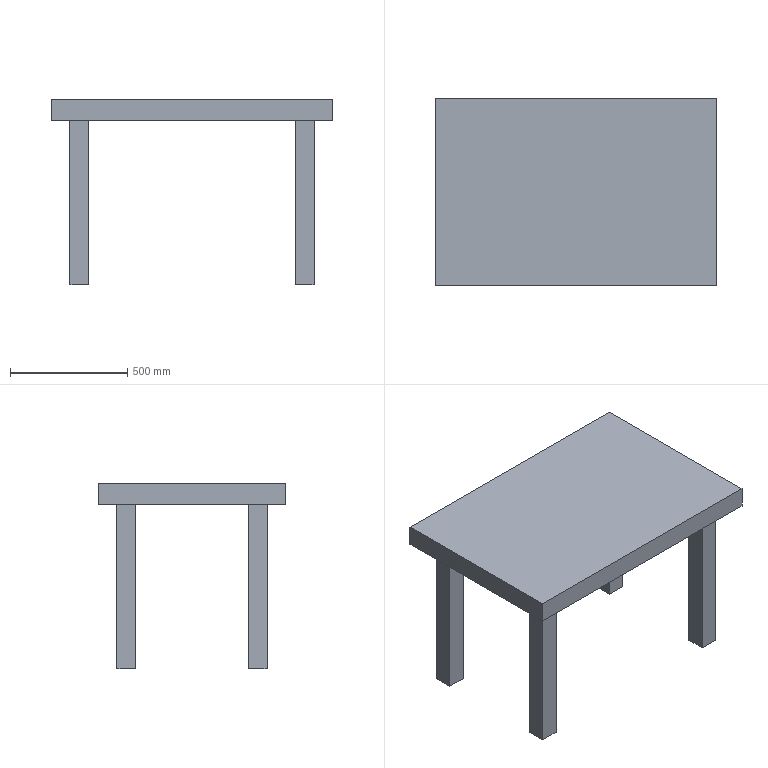Part | SolidWorks | features MirrorPattern 2, Extrusion 1, ICE 1 | 1 solid | 26 faces | box 1200 x 800 x 790 mm | volume 104320000 mm3 | plane 26
STEP:
#1=CARTESIAN_POINT('',(440.,-320.,-90.));
#2=VERTEX_POINT('',#1);
#3=CARTESIAN_POINT('',(520.,-320.,-90.));
#4=VERTEX_POINT('',#3);
#5=CARTESIAN_POINT('',(520.,-320.,-90.));
#6=DIRECTION('',(1.,0.,0.));
#7=VECTOR('',#6,1000.);
#8=LINE('',#5,#7);
#9=EDGE_CURVE('',#2,#4,#8,.T.);
#10=ORIENTED_EDGE('',*,*,#9,.T.);
#11=CARTESIAN_POINT('',(520.,-240.,-90.));
#12=VERTEX_POINT('',#11);
#13=CARTESIAN_POINT('',(520.,-320.,-90.));
#14=DIRECTION('',(0.,1.,0.));
#15=VECTOR('',#14,1000.);
#16=LINE('',#13,#15);
#17=EDGE_CURVE('',#4,#12,#16,.T.);
#18=ORIENTED_EDGE('',*,*,#17,.T.);
#19=CARTESIAN_POINT('',(440.,-240.,-90.));
#20=VERTEX_POINT('',#19);
#21=CARTESIAN_POINT('',(520.,-240.,-90.));
#22=DIRECTION('',(-1.,0.,0.));
#23=VECTOR('',#22,1000.);
#24=LINE('',#21,#23);
#25=EDGE_CURVE('',#12,#20,#24,.T.);
#26=ORIENTED_EDGE('',*,*,#25,.T.);
#27=CARTESIAN_POINT('',(440.,-320.,-90.));
#28=DIRECTION('',(0.,-1.,0.));
#29=VECTOR('',#28,1000.);
#30=LINE('',#27,#29);
#31=EDGE_CURVE('',#20,#2,#30,.T.);
#32=ORIENTED_EDGE('',*,*,#31,.T.);
#33=EDGE_LOOP('',(#10,#18,#26,#32));
#34=FACE_BOUND('',#33,.T.);
#35=CARTESIAN_POINT('',(-520.,-320.,-90.));
#36=VERTEX_POINT('',#35);
#37=CARTESIAN_POINT('',(-520.,-240.,-90.));
#38=VERTEX_POINT('',#37);
#39=CARTESIAN_POINT('',(-520.,-320.,-90.));
#40=DIRECTION('',(0.,1.,0.));
#41=VECTOR('',#40,1000.);
#42=LINE('',#39,#41);
#43=EDGE_CURVE('',#36,#38,#42,.T.);
#44=ORIENTED_EDGE('',*,*,#43,.F.);
#45=CARTESIAN_POINT('',(-440.,-320.,-90.));
#46=VERTEX_POINT('',#45);
#47=CARTESIAN_POINT('',(-520.,-320.,-90.));
#48=DIRECTION('',(-1.,0.,0.));
#49=VECTOR('',#48,1000.);
#50=LINE('',#47,#49);
#51=EDGE_CURVE('',#46,#36,#50,.T.);
#52=ORIENTED_EDGE('',*,*,#51,.F.);
#53=CARTESIAN_POINT('',(-440.,-240.,-90.));
#54=VERTEX_POINT('',#53);
#55=CARTESIAN_POINT('',(-440.,-320.,-90.));
#56=DIRECTION('',(0.,-1.,0.));
#57=VECTOR('',#56,1000.);
#58=LINE('',#55,#57);
#59=EDGE_CURVE('',#54,#46,#58,.T.);
#60=ORIENTED_EDGE('',*,*,#59,.F.);
#61=CARTESIAN_POINT('',(-520.,-240.,-90.));
#62=DIRECTION('',(1.,0.,0.));
#63=VECTOR('',#62,1000.);
#64=LINE('',#61,#63);
#65=EDGE_CURVE('',#38,#54,#64,.T.);
#66=ORIENTED_EDGE('',*,*,#65,.F.);
#67=EDGE_LOOP('',(#44,#52,#60,#66));
#68=FACE_BOUND('',#67,.T.);
#69=CARTESIAN_POINT('',(-600.,400.,-90.));
#70=VERTEX_POINT('',#69);
#71=CARTESIAN_POINT('',(-600.,-400.,-90.));
#72=VERTEX_POINT('',#71);
#73=CARTESIAN_POINT('',(-600.,-400.,-90.));
#74=DIRECTION('',(0.,-1.,0.));
#75=VECTOR('',#74,1000.);
#76=LINE('',#73,#75);
#77=EDGE_CURVE('',#70,#72,#76,.T.);
#78=ORIENTED_EDGE('',*,*,#77,.F.);
#79=CARTESIAN_POINT('',(600.,400.,-90.));
#80=VERTEX_POINT('',#79);
#81=CARTESIAN_POINT('',(600.,400.,-90.));
#82=DIRECTION('',(-1.,0.,0.));
#83=VECTOR('',#82,1000.);
#84=LINE('',#81,#83);
#85=EDGE_CURVE('',#80,#70,#84,.T.);
#86=ORIENTED_EDGE('',*,*,#85,.F.);
#87=CARTESIAN_POINT('',(600.,-400.,-90.));
#88=VERTEX_POINT('',#87);
#89=CARTESIAN_POINT('',(600.,-400.,-90.));
#90=DIRECTION('',(0.,1.,0.));
#91=VECTOR('',#90,1000.);
#92=LINE('',#89,#91);
#93=EDGE_CURVE('',#88,#80,#92,.T.);
#94=ORIENTED_EDGE('',*,*,#93,.F.);
#95=CARTESIAN_POINT('',(600.,-400.,-90.));
#96=DIRECTION('',(1.,0.,0.));
#97=VECTOR('',#96,1000.);
#98=LINE('',#95,#97);
#99=EDGE_CURVE('',#72,#88,#98,.T.);
#100=ORIENTED_EDGE('',*,*,#99,.F.);
#101=EDGE_LOOP('',(#78,#86,#94,#100));
#102=FACE_OUTER_BOUND('',#101,.T.);
#103=CARTESIAN_POINT('',(-440.,320.,-90.));
#104=VERTEX_POINT('',#103);
#105=CARTESIAN_POINT('',(-520.,320.,-90.));
#106=VERTEX_POINT('',#105);
#107=CARTESIAN_POINT('',(-520.,320.,-90.));
#108=DIRECTION('',(-1.,0.,0.));
#109=VECTOR('',#108,1000.);
#110=LINE('',#107,#109);
#111=EDGE_CURVE('',#104,#106,#110,.T.);
#112=ORIENTED_EDGE('',*,*,#111,.T.);
#113=CARTESIAN_POINT('',(-520.,240.,-90.));
#114=VERTEX_POINT('',#113);
#115=CARTESIAN_POINT('',(-520.,320.,-90.));
#116=DIRECTION('',(0.,-1.,0.));
#117=VECTOR('',#116,1000.);
#118=LINE('',#115,#117);
#119=EDGE_CURVE('',#106,#114,#118,.T.);
#120=ORIENTED_EDGE('',*,*,#119,.T.);
#121=CARTESIAN_POINT('',(-440.,240.,-90.));
#122=VERTEX_POINT('',#121);
#123=CARTESIAN_POINT('',(-520.,240.,-90.));
#124=DIRECTION('',(1.,0.,0.));
#125=VECTOR('',#124,1000.);
#126=LINE('',#123,#125);
#127=EDGE_CURVE('',#114,#122,#126,.T.);
#128=ORIENTED_EDGE('',*,*,#127,.T.);
#129=CARTESIAN_POINT('',(-440.,320.,-90.));
#130=DIRECTION('',(0.,1.,0.));
#131=VECTOR('',#130,1000.);
#132=LINE('',#129,#131);
#133=EDGE_CURVE('',#122,#104,#132,.T.);
#134=ORIENTED_EDGE('',*,*,#133,.T.);
#135=EDGE_LOOP('',(#112,#120,#128,#134));
#136=FACE_BOUND('',#135,.T.);
#137=CARTESIAN_POINT('',(520.,320.,-90.));
#138=VERTEX_POINT('',#137);
#139=CARTESIAN_POINT('',(520.,240.,-90.));
#140=VERTEX_POINT('',#139);
#141=CARTESIAN_POINT('',(520.,320.,-90.));
#142=DIRECTION('',(0.,-1.,0.));
#143=VECTOR('',#142,1000.);
#144=LINE('',#141,#143);
#145=EDGE_CURVE('',#138,#140,#144,.T.);
#146=ORIENTED_EDGE('',*,*,#145,.F.);
#147=CARTESIAN_POINT('',(440.,320.,-90.));
#148=VERTEX_POINT('',#147);
#149=CARTESIAN_POINT('',(520.,320.,-90.));
#150=DIRECTION('',(1.,0.,0.));
#151=VECTOR('',#150,1000.);
#152=LINE('',#149,#151);
#153=EDGE_CURVE('',#148,#138,#152,.T.);
#154=ORIENTED_EDGE('',*,*,#153,.F.);
#155=CARTESIAN_POINT('',(440.,240.,-90.));
#156=VERTEX_POINT('',#155);
#157=CARTESIAN_POINT('',(440.,320.,-90.));
#158=DIRECTION('',(0.,1.,0.));
#159=VECTOR('',#158,1000.);
#160=LINE('',#157,#159);
#161=EDGE_CURVE('',#156,#148,#160,.T.);
#162=ORIENTED_EDGE('',*,*,#161,.F.);
#163=CARTESIAN_POINT('',(520.,240.,-90.));
#164=DIRECTION('',(-1.,0.,0.));
#165=VECTOR('',#164,1000.);
#166=LINE('',#163,#165);
#167=EDGE_CURVE('',#140,#156,#166,.T.);
#168=ORIENTED_EDGE('',*,*,#167,.F.);
#169=EDGE_LOOP('',(#146,#154,#162,#168));
#170=FACE_BOUND('',#169,.T.);
#171=CARTESIAN_POINT('',(0.,0.,-90.));
#172=DIRECTION('',(0.,0.,1.));
#173=DIRECTION('',(1.,0.,0.));
#174=AXIS2_PLACEMENT_3D('',#171,#172,#173);
#175=PLANE('',#174);
#176=ADVANCED_FACE('',(#34,#68,#102,#136,#170),#175,.F.);
#177=CARTESIAN_POINT('',(-600.,400.,0.));
#178=VERTEX_POINT('',#177);
#179=CARTESIAN_POINT('',(-600.,-400.,0.));
#180=VERTEX_POINT('',#179);
#181=CARTESIAN_POINT('',(-600.,-400.,0.));
#182=DIRECTION('',(0.,-1.,0.));
#183=VECTOR('',#182,1000.);
#184=LINE('',#181,#183);
#185=EDGE_CURVE('',#178,#180,#184,.T.);
#186=ORIENTED_EDGE('',*,*,#185,.F.);
#187=CARTESIAN_POINT('',(-600.,400.,-90.));
#188=DIRECTION('',(0.,0.,1.));
#189=VECTOR('',#188,1000.);
#190=LINE('',#187,#189);
#191=EDGE_CURVE('',#70,#178,#190,.T.);
#192=ORIENTED_EDGE('',*,*,#191,.F.);
#193=ORIENTED_EDGE('',*,*,#77,.T.);
#194=CARTESIAN_POINT('',(-600.,-400.,-90.));
#195=DIRECTION('',(0.,0.,1.));
#196=VECTOR('',#195,1000.);
#197=LINE('',#194,#196);
#198=EDGE_CURVE('',#72,#180,#197,.T.);
#199=ORIENTED_EDGE('',*,*,#198,.T.);
#200=EDGE_LOOP('',(#186,#192,#193,#199));
#201=FACE_OUTER_BOUND('',#200,.T.);
#202=CARTESIAN_POINT('',(-600.,-400.,-90.));
#203=DIRECTION('',(-1.,0.,0.));
#204=DIRECTION('',(0.,0.,1.));
#205=AXIS2_PLACEMENT_3D('',#202,#203,#204);
#206=PLANE('',#205);
#207=ADVANCED_FACE('',(#201),#206,.T.);
#208=CARTESIAN_POINT('',(600.,400.,0.));
#209=VERTEX_POINT('',#208);
#210=CARTESIAN_POINT('',(600.,400.,0.));
#211=DIRECTION('',(-1.,0.,0.));
#212=VECTOR('',#211,1000.);
#213=LINE('',#210,#212);
#214=EDGE_CURVE('',#209,#178,#213,.T.);
#215=ORIENTED_EDGE('',*,*,#214,.F.);
#216=CARTESIAN_POINT('',(600.,400.,-90.));
#217=DIRECTION('',(0.,0.,1.));
#218=VECTOR('',#217,1000.);
#219=LINE('',#216,#218);
#220=EDGE_CURVE('',#80,#209,#219,.T.);
#221=ORIENTED_EDGE('',*,*,#220,.F.);
#222=ORIENTED_EDGE('',*,*,#85,.T.);
#223=ORIENTED_EDGE('',*,*,#191,.T.);
#224=EDGE_LOOP('',(#215,#221,#222,#223));
#225=FACE_OUTER_BOUND('',#224,.T.);
#226=CARTESIAN_POINT('',(600.,400.,-90.));
#227=DIRECTION('',(0.,1.,0.));
#228=DIRECTION('',(-1.,0.,0.));
#229=AXIS2_PLACEMENT_3D('',#226,#227,#228);
#230=PLANE('',#229);
#231=ADVANCED_FACE('',(#225),#230,.T.);
#232=CARTESIAN_POINT('',(600.,-400.,0.));
#233=VERTEX_POINT('',#232);
#234=CARTESIAN_POINT('',(600.,-400.,0.));
#235=DIRECTION('',(0.,1.,0.));
#236=VECTOR('',#235,1000.);
#237=LINE('',#234,#236);
#238=EDGE_CURVE('',#233,#209,#237,.T.);
#239=ORIENTED_EDGE('',*,*,#238,.F.);
#240=CARTESIAN_POINT('',(600.,-400.,-90.));
#241=DIRECTION('',(0.,0.,1.));
#242=VECTOR('',#241,1000.);
#243=LINE('',#240,#242);
#244=EDGE_CURVE('',#88,#233,#243,.T.);
#245=ORIENTED_EDGE('',*,*,#244,.F.);
#246=ORIENTED_EDGE('',*,*,#93,.T.);
#247=ORIENTED_EDGE('',*,*,#220,.T.);
#248=EDGE_LOOP('',(#239,#245,#246,#247));
#249=FACE_OUTER_BOUND('',#248,.T.);
#250=CARTESIAN_POINT('',(600.,-400.,-90.));
#251=DIRECTION('',(1.,0.,0.));
#252=DIRECTION('',(0.,0.,-1.));
#253=AXIS2_PLACEMENT_3D('',#250,#251,#252);
#254=PLANE('',#253);
#255=ADVANCED_FACE('',(#249),#254,.T.);
#256=CARTESIAN_POINT('',(600.,-400.,0.));
#257=DIRECTION('',(1.,0.,0.));
#258=VECTOR('',#257,1000.);
#259=LINE('',#256,#258);
#260=EDGE_CURVE('',#180,#233,#259,.T.);
#261=ORIENTED_EDGE('',*,*,#260,.F.);
#262=ORIENTED_EDGE('',*,*,#198,.F.);
#263=ORIENTED_EDGE('',*,*,#99,.T.);
#264=ORIENTED_EDGE('',*,*,#244,.T.);
#265=EDGE_LOOP('',(#261,#262,#263,#264));
#266=FACE_OUTER_BOUND('',#265,.T.);
#267=CARTESIAN_POINT('',(600.,-400.,-90.));
#268=DIRECTION('',(0.,-1.,0.));
#269=DIRECTION('',(1.,0.,0.));
#270=AXIS2_PLACEMENT_3D('',#267,#268,#269);
#271=PLANE('',#270);
#272=ADVANCED_FACE('',(#266),#271,.T.);
#273=ORIENTED_EDGE('',*,*,#185,.T.);
#274=ORIENTED_EDGE('',*,*,#260,.T.);
#275=ORIENTED_EDGE('',*,*,#238,.T.);
#276=ORIENTED_EDGE('',*,*,#214,.T.);
#277=EDGE_LOOP('',(#273,#274,#275,#276));
#278=FACE_OUTER_BOUND('',#277,.T.);
#279=CARTESIAN_POINT('',(0.,0.,0.));
#280=DIRECTION('',(0.,0.,1.));
#281=DIRECTION('',(1.,0.,0.));
#282=AXIS2_PLACEMENT_3D('',#279,#280,#281);
#283=PLANE('',#282);
#284=ADVANCED_FACE('',(#278),#283,.T.);
#285=ORIENTED_EDGE('',*,*,#43,.T.);
#286=CARTESIAN_POINT('',(-520.,-240.,-790.));
#287=VERTEX_POINT('',#286);
#288=CARTESIAN_POINT('',(-520.,-240.,-790.));
#289=DIRECTION('',(0.,0.,1.));
#290=VECTOR('',#289,1000.);
#291=LINE('',#288,#290);
#292=EDGE_CURVE('',#287,#38,#291,.T.);
#293=ORIENTED_EDGE('',*,*,#292,.F.);
#294=CARTESIAN_POINT('',(-520.,-320.,-790.));
#295=VERTEX_POINT('',#294);
#296=CARTESIAN_POINT('',(-520.,-320.,-790.));
#297=DIRECTION('',(0.,1.,0.));
#298=VECTOR('',#297,1000.);
#299=LINE('',#296,#298);
#300=EDGE_CURVE('',#295,#287,#299,.T.);
#301=ORIENTED_EDGE('',*,*,#300,.F.);
#302=CARTESIAN_POINT('',(-520.,-320.,-790.));
#303=DIRECTION('',(0.,0.,1.));
#304=VECTOR('',#303,1000.);
#305=LINE('',#302,#304);
#306=EDGE_CURVE('',#295,#36,#305,.T.);
#307=ORIENTED_EDGE('',*,*,#306,.T.);
#308=EDGE_LOOP('',(#285,#293,#301,#307));
#309=FACE_OUTER_BOUND('',#308,.T.);
#310=CARTESIAN_POINT('',(-520.,-320.,-790.));
#311=DIRECTION('',(1.,0.,0.));
#312=DIRECTION('',(0.,0.,-1.));
#313=AXIS2_PLACEMENT_3D('',#310,#311,#312);
#314=PLANE('',#313);
#315=ADVANCED_FACE('',(#309),#314,.F.);
#316=ORIENTED_EDGE('',*,*,#65,.T.);
#317=CARTESIAN_POINT('',(-440.,-240.,-790.));
#318=VERTEX_POINT('',#317);
#319=CARTESIAN_POINT('',(-440.,-240.,-790.));
#320=DIRECTION('',(0.,0.,1.));
#321=VECTOR('',#320,1000.);
#322=LINE('',#319,#321);
#323=EDGE_CURVE('',#318,#54,#322,.T.);
#324=ORIENTED_EDGE('',*,*,#323,.F.);
#325=CARTESIAN_POINT('',(-520.,-240.,-790.));
#326=DIRECTION('',(1.,0.,0.));
#327=VECTOR('',#326,1000.);
#328=LINE('',#325,#327);
#329=EDGE_CURVE('',#287,#318,#328,.T.);
#330=ORIENTED_EDGE('',*,*,#329,.F.);
#331=ORIENTED_EDGE('',*,*,#292,.T.);
#332=EDGE_LOOP('',(#316,#324,#330,#331));
#333=FACE_OUTER_BOUND('',#332,.T.);
#334=CARTESIAN_POINT('',(-520.,-240.,-790.));
#335=DIRECTION('',(0.,-1.,0.));
#336=DIRECTION('',(0.,0.,-1.));
#337=AXIS2_PLACEMENT_3D('',#334,#335,#336);
#338=PLANE('',#337);
#339=ADVANCED_FACE('',(#333),#338,.F.);
#340=ORIENTED_EDGE('',*,*,#59,.T.);
#341=CARTESIAN_POINT('',(-440.,-320.,-790.));
#342=VERTEX_POINT('',#341);
#343=CARTESIAN_POINT('',(-440.,-320.,-790.));
#344=DIRECTION('',(0.,0.,1.));
#345=VECTOR('',#344,1000.);
#346=LINE('',#343,#345);
#347=EDGE_CURVE('',#342,#46,#346,.T.);
#348=ORIENTED_EDGE('',*,*,#347,.F.);
#349=CARTESIAN_POINT('',(-440.,-320.,-790.));
#350=DIRECTION('',(0.,-1.,0.));
#351=VECTOR('',#350,1000.);
#352=LINE('',#349,#351);
#353=EDGE_CURVE('',#318,#342,#352,.T.);
#354=ORIENTED_EDGE('',*,*,#353,.F.);
#355=ORIENTED_EDGE('',*,*,#323,.T.);
#356=EDGE_LOOP('',(#340,#348,#354,#355));
#357=FACE_OUTER_BOUND('',#356,.T.);
#358=CARTESIAN_POINT('',(-440.,-320.,-790.));
#359=DIRECTION('',(-1.,0.,0.));
#360=DIRECTION('',(0.,0.,1.));
#361=AXIS2_PLACEMENT_3D('',#358,#359,#360);
#362=PLANE('',#361);
#363=ADVANCED_FACE('',(#357),#362,.F.);
#364=ORIENTED_EDGE('',*,*,#51,.T.);
#365=ORIENTED_EDGE('',*,*,#306,.F.);
#366=CARTESIAN_POINT('',(-520.,-320.,-790.));
#367=DIRECTION('',(-1.,0.,0.));
#368=VECTOR('',#367,1000.);
#369=LINE('',#366,#368);
#370=EDGE_CURVE('',#342,#295,#369,.T.);
#371=ORIENTED_EDGE('',*,*,#370,.F.);
#372=ORIENTED_EDGE('',*,*,#347,.T.);
#373=EDGE_LOOP('',(#364,#365,#371,#372));
#374=FACE_OUTER_BOUND('',#373,.T.);
#375=CARTESIAN_POINT('',(-520.,-320.,-790.));
#376=DIRECTION('',(0.,1.,0.));
#377=DIRECTION('',(0.,0.,1.));
#378=AXIS2_PLACEMENT_3D('',#375,#376,#377);
#379=PLANE('',#378);
#380=ADVANCED_FACE('',(#374),#379,.F.);
#381=ORIENTED_EDGE('',*,*,#300,.T.);
#382=ORIENTED_EDGE('',*,*,#329,.T.);
#383=ORIENTED_EDGE('',*,*,#353,.T.);
#384=ORIENTED_EDGE('',*,*,#370,.T.);
#385=EDGE_LOOP('',(#381,#382,#383,#384));
#386=FACE_OUTER_BOUND('',#385,.T.);
#387=CARTESIAN_POINT('',(0.,0.,-790.));
#388=DIRECTION('',(0.,0.,-1.));
#389=DIRECTION('',(-1.,0.,0.));
#390=AXIS2_PLACEMENT_3D('',#387,#388,#389);
#391=PLANE('',#390);
#392=ADVANCED_FACE('',(#386),#391,.T.);
#393=ORIENTED_EDGE('',*,*,#119,.F.);
#394=CARTESIAN_POINT('',(-520.,320.,-790.));
#395=VERTEX_POINT('',#394);
#396=CARTESIAN_POINT('',(-520.,320.,-790.));
#397=DIRECTION('',(0.,0.,1.));
#398=VECTOR('',#397,1000.);
#399=LINE('',#396,#398);
#400=EDGE_CURVE('',#395,#106,#399,.T.);
#401=ORIENTED_EDGE('',*,*,#400,.F.);
#402=CARTESIAN_POINT('',(-520.,240.,-790.));
#403=VERTEX_POINT('',#402);
#404=CARTESIAN_POINT('',(-520.,320.,-790.));
#405=DIRECTION('',(0.,-1.,0.));
#406=VECTOR('',#405,1000.);
#407=LINE('',#404,#406);
#408=EDGE_CURVE('',#395,#403,#407,.T.);
#409=ORIENTED_EDGE('',*,*,#408,.T.);
#410=CARTESIAN_POINT('',(-520.,240.,-790.));
#411=DIRECTION('',(0.,0.,1.));
#412=VECTOR('',#411,1000.);
#413=LINE('',#410,#412);
#414=EDGE_CURVE('',#403,#114,#413,.T.);
#415=ORIENTED_EDGE('',*,*,#414,.T.);
#416=EDGE_LOOP('',(#393,#401,#409,#415));
#417=FACE_OUTER_BOUND('',#416,.T.);
#418=CARTESIAN_POINT('',(-520.,320.,-790.));
#419=DIRECTION('',(-1.,0.,0.));
#420=DIRECTION('',(0.,0.,1.));
#421=AXIS2_PLACEMENT_3D('',#418,#419,#420);
#422=PLANE('',#421);
#423=ADVANCED_FACE('',(#417),#422,.T.);
#424=ORIENTED_EDGE('',*,*,#111,.F.);
#425=CARTESIAN_POINT('',(-440.,320.,-790.));
#426=VERTEX_POINT('',#425);
#427=CARTESIAN_POINT('',(-440.,320.,-790.));
#428=DIRECTION('',(0.,0.,1.));
#429=VECTOR('',#428,1000.);
#430=LINE('',#427,#429);
#431=EDGE_CURVE('',#426,#104,#430,.T.);
#432=ORIENTED_EDGE('',*,*,#431,.F.);
#433=CARTESIAN_POINT('',(-520.,320.,-790.));
#434=DIRECTION('',(-1.,0.,0.));
#435=VECTOR('',#434,1000.);
#436=LINE('',#433,#435);
#437=EDGE_CURVE('',#426,#395,#436,.T.);
#438=ORIENTED_EDGE('',*,*,#437,.T.);
#439=ORIENTED_EDGE('',*,*,#400,.T.);
#440=EDGE_LOOP('',(#424,#432,#438,#439));
#441=FACE_OUTER_BOUND('',#440,.T.);
#442=CARTESIAN_POINT('',(-520.,320.,-790.));
#443=DIRECTION('',(0.,1.,0.));
#444=DIRECTION('',(0.,0.,1.));
#445=AXIS2_PLACEMENT_3D('',#442,#443,#444);
#446=PLANE('',#445);
#447=ADVANCED_FACE('',(#441),#446,.T.);
#448=ORIENTED_EDGE('',*,*,#133,.F.);
#449=CARTESIAN_POINT('',(-440.,240.,-790.));
#450=VERTEX_POINT('',#449);
#451=CARTESIAN_POINT('',(-440.,240.,-790.));
#452=DIRECTION('',(0.,0.,1.));
#453=VECTOR('',#452,1000.);
#454=LINE('',#451,#453);
#455=EDGE_CURVE('',#450,#122,#454,.T.);
#456=ORIENTED_EDGE('',*,*,#455,.F.);
#457=CARTESIAN_POINT('',(-440.,320.,-790.));
#458=DIRECTION('',(0.,1.,0.));
#459=VECTOR('',#458,1000.);
#460=LINE('',#457,#459);
#461=EDGE_CURVE('',#450,#426,#460,.T.);
#462=ORIENTED_EDGE('',*,*,#461,.T.);
#463=ORIENTED_EDGE('',*,*,#431,.T.);
#464=EDGE_LOOP('',(#448,#456,#462,#463));
#465=FACE_OUTER_BOUND('',#464,.T.);
#466=CARTESIAN_POINT('',(-440.,320.,-790.));
#467=DIRECTION('',(1.,0.,0.));
#468=DIRECTION('',(0.,0.,-1.));
#469=AXIS2_PLACEMENT_3D('',#466,#467,#468);
#470=PLANE('',#469);
#471=ADVANCED_FACE('',(#465),#470,.T.);
#472=ORIENTED_EDGE('',*,*,#127,.F.);
#473=ORIENTED_EDGE('',*,*,#414,.F.);
#474=CARTESIAN_POINT('',(-520.,240.,-790.));
#475=DIRECTION('',(1.,0.,0.));
#476=VECTOR('',#475,1000.);
#477=LINE('',#474,#476);
#478=EDGE_CURVE('',#403,#450,#477,.T.);
#479=ORIENTED_EDGE('',*,*,#478,.T.);
#480=ORIENTED_EDGE('',*,*,#455,.T.);
#481=EDGE_LOOP('',(#472,#473,#479,#480));
#482=FACE_OUTER_BOUND('',#481,.T.);
#483=CARTESIAN_POINT('',(-520.,240.,-790.));
#484=DIRECTION('',(0.,-1.,0.));
#485=DIRECTION('',(0.,0.,-1.));
#486=AXIS2_PLACEMENT_3D('',#483,#484,#485);
#487=PLANE('',#486);
#488=ADVANCED_FACE('',(#482),#487,.T.);
#489=ORIENTED_EDGE('',*,*,#408,.F.);
#490=ORIENTED_EDGE('',*,*,#437,.F.);
#491=ORIENTED_EDGE('',*,*,#461,.F.);
#492=ORIENTED_EDGE('',*,*,#478,.F.);
#493=EDGE_LOOP('',(#489,#490,#491,#492));
#494=FACE_OUTER_BOUND('',#493,.T.);
#495=CARTESIAN_POINT('',(0.,0.,-790.));
#496=DIRECTION('',(0.,0.,-1.));
#497=DIRECTION('',(-1.,0.,0.));
#498=AXIS2_PLACEMENT_3D('',#495,#496,#497);
#499=PLANE('',#498);
#500=ADVANCED_FACE('',(#494),#499,.T.);
#501=ORIENTED_EDGE('',*,*,#145,.T.);
#502=CARTESIAN_POINT('',(520.,240.,-790.));
#503=VERTEX_POINT('',#502);
#504=CARTESIAN_POINT('',(520.,240.,-790.));
#505=DIRECTION('',(0.,0.,1.));
#506=VECTOR('',#505,1000.);
#507=LINE('',#504,#506);
#508=EDGE_CURVE('',#503,#140,#507,.T.);
#509=ORIENTED_EDGE('',*,*,#508,.F.);
#510=CARTESIAN_POINT('',(520.,320.,-790.));
#511=VERTEX_POINT('',#510);
#512=CARTESIAN_POINT('',(520.,320.,-790.));
#513=DIRECTION('',(0.,-1.,0.));
#514=VECTOR('',#513,1000.);
#515=LINE('',#512,#514);
#516=EDGE_CURVE('',#511,#503,#515,.T.);
#517=ORIENTED_EDGE('',*,*,#516,.F.);
#518=CARTESIAN_POINT('',(520.,320.,-790.));
#519=DIRECTION('',(0.,0.,1.));
#520=VECTOR('',#519,1000.);
#521=LINE('',#518,#520);
#522=EDGE_CURVE('',#511,#138,#521,.T.);
#523=ORIENTED_EDGE('',*,*,#522,.T.);
#524=EDGE_LOOP('',(#501,#509,#517,#523));
#525=FACE_OUTER_BOUND('',#524,.T.);
#526=CARTESIAN_POINT('',(520.,320.,-790.));
#527=DIRECTION('',(-1.,0.,0.));
#528=DIRECTION('',(0.,0.,1.));
#529=AXIS2_PLACEMENT_3D('',#526,#527,#528);
#530=PLANE('',#529);
#531=ADVANCED_FACE('',(#525),#530,.F.);
#532=ORIENTED_EDGE('',*,*,#167,.T.);
#533=CARTESIAN_POINT('',(440.,240.,-790.));
#534=VERTEX_POINT('',#533);
#535=CARTESIAN_POINT('',(440.,240.,-790.));
#536=DIRECTION('',(0.,0.,1.));
#537=VECTOR('',#536,1000.);
#538=LINE('',#535,#537);
#539=EDGE_CURVE('',#534,#156,#538,.T.);
#540=ORIENTED_EDGE('',*,*,#539,.F.);
#541=CARTESIAN_POINT('',(520.,240.,-790.));
#542=DIRECTION('',(-1.,0.,0.));
#543=VECTOR('',#542,1000.);
#544=LINE('',#541,#543);
#545=EDGE_CURVE('',#503,#534,#544,.T.);
#546=ORIENTED_EDGE('',*,*,#545,.F.);
#547=ORIENTED_EDGE('',*,*,#508,.T.);
#548=EDGE_LOOP('',(#532,#540,#546,#547));
#549=FACE_OUTER_BOUND('',#548,.T.);
#550=CARTESIAN_POINT('',(520.,240.,-790.));
#551=DIRECTION('',(0.,1.,0.));
#552=DIRECTION('',(0.,0.,1.));
#553=AXIS2_PLACEMENT_3D('',#550,#551,#552);
#554=PLANE('',#553);
#555=ADVANCED_FACE('',(#549),#554,.F.);
#556=ORIENTED_EDGE('',*,*,#161,.T.);
#557=CARTESIAN_POINT('',(440.,320.,-790.));
#558=VERTEX_POINT('',#557);
#559=CARTESIAN_POINT('',(440.,320.,-790.));
#560=DIRECTION('',(0.,0.,1.));
#561=VECTOR('',#560,1000.);
#562=LINE('',#559,#561);
#563=EDGE_CURVE('',#558,#148,#562,.T.);
#564=ORIENTED_EDGE('',*,*,#563,.F.);
#565=CARTESIAN_POINT('',(440.,320.,-790.));
#566=DIRECTION('',(0.,1.,0.));
#567=VECTOR('',#566,1000.);
#568=LINE('',#565,#567);
#569=EDGE_CURVE('',#534,#558,#568,.T.);
#570=ORIENTED_EDGE('',*,*,#569,.F.);
#571=ORIENTED_EDGE('',*,*,#539,.T.);
#572=EDGE_LOOP('',(#556,#564,#570,#571));
#573=FACE_OUTER_BOUND('',#572,.T.);
#574=CARTESIAN_POINT('',(440.,320.,-790.));
#575=DIRECTION('',(1.,0.,0.));
#576=DIRECTION('',(0.,0.,-1.));
#577=AXIS2_PLACEMENT_3D('',#574,#575,#576);
#578=PLANE('',#577);
#579=ADVANCED_FACE('',(#573),#578,.F.);
#580=ORIENTED_EDGE('',*,*,#153,.T.);
#581=ORIENTED_EDGE('',*,*,#522,.F.);
#582=CARTESIAN_POINT('',(520.,320.,-790.));
#583=DIRECTION('',(1.,0.,0.));
#584=VECTOR('',#583,1000.);
#585=LINE('',#582,#584);
#586=EDGE_CURVE('',#558,#511,#585,.T.);
#587=ORIENTED_EDGE('',*,*,#586,.F.);
#588=ORIENTED_EDGE('',*,*,#563,.T.);
#589=EDGE_LOOP('',(#580,#581,#587,#588));
#590=FACE_OUTER_BOUND('',#589,.T.);
#591=CARTESIAN_POINT('',(520.,320.,-790.));
#592=DIRECTION('',(0.,-1.,0.));
#593=DIRECTION('',(0.,0.,-1.));
#594=AXIS2_PLACEMENT_3D('',#591,#592,#593);
#595=PLANE('',#594);
#596=ADVANCED_FACE('',(#590),#595,.F.);
#597=ORIENTED_EDGE('',*,*,#516,.T.);
#598=ORIENTED_EDGE('',*,*,#545,.T.);
#599=ORIENTED_EDGE('',*,*,#569,.T.);
#600=ORIENTED_EDGE('',*,*,#586,.T.);
#601=EDGE_LOOP('',(#597,#598,#599,#600));
#602=FACE_OUTER_BOUND('',#601,.T.);
#603=CARTESIAN_POINT('',(0.,0.,-790.));
#604=DIRECTION('',(0.,0.,-1.));
#605=DIRECTION('',(1.,0.,0.));
#606=AXIS2_PLACEMENT_3D('',#603,#604,#605);
#607=PLANE('',#606);
#608=ADVANCED_FACE('',(#602),#607,.T.);
#609=ORIENTED_EDGE('',*,*,#17,.F.);
#610=CARTESIAN_POINT('',(520.,-320.,-790.));
#611=VERTEX_POINT('',#610);
#612=CARTESIAN_POINT('',(520.,-320.,-790.));
#613=DIRECTION('',(0.,0.,1.));
#614=VECTOR('',#613,1000.);
#615=LINE('',#612,#614);
#616=EDGE_CURVE('',#611,#4,#615,.T.);
#617=ORIENTED_EDGE('',*,*,#616,.F.);
#618=CARTESIAN_POINT('',(520.,-240.,-790.));
#619=VERTEX_POINT('',#618);
#620=CARTESIAN_POINT('',(520.,-320.,-790.));
#621=DIRECTION('',(0.,1.,0.));
#622=VECTOR('',#621,1000.);
#623=LINE('',#620,#622);
#624=EDGE_CURVE('',#611,#619,#623,.T.);
#625=ORIENTED_EDGE('',*,*,#624,.T.);
#626=CARTESIAN_POINT('',(520.,-240.,-790.));
#627=DIRECTION('',(0.,0.,1.));
#628=VECTOR('',#627,1000.);
#629=LINE('',#626,#628);
#630=EDGE_CURVE('',#619,#12,#629,.T.);
#631=ORIENTED_EDGE('',*,*,#630,.T.);
#632=EDGE_LOOP('',(#609,#617,#625,#631));
#633=FACE_OUTER_BOUND('',#632,.T.);
#634=CARTESIAN_POINT('',(520.,-320.,-790.));
#635=DIRECTION('',(1.,0.,0.));
#636=DIRECTION('',(0.,0.,-1.));
#637=AXIS2_PLACEMENT_3D('',#634,#635,#636);
#638=PLANE('',#637);
#639=ADVANCED_FACE('',(#633),#638,.T.);
#640=ORIENTED_EDGE('',*,*,#9,.F.);
#641=CARTESIAN_POINT('',(440.,-320.,-790.));
#642=VERTEX_POINT('',#641);
#643=CARTESIAN_POINT('',(440.,-320.,-790.));
#644=DIRECTION('',(0.,0.,1.));
#645=VECTOR('',#644,1000.);
#646=LINE('',#643,#645);
#647=EDGE_CURVE('',#642,#2,#646,.T.);
#648=ORIENTED_EDGE('',*,*,#647,.F.);
#649=CARTESIAN_POINT('',(520.,-320.,-790.));
#650=DIRECTION('',(1.,0.,0.));
#651=VECTOR('',#650,1000.);
#652=LINE('',#649,#651);
#653=EDGE_CURVE('',#642,#611,#652,.T.);
#654=ORIENTED_EDGE('',*,*,#653,.T.);
#655=ORIENTED_EDGE('',*,*,#616,.T.);
#656=EDGE_LOOP('',(#640,#648,#654,#655));
#657=FACE_OUTER_BOUND('',#656,.T.);
#658=CARTESIAN_POINT('',(520.,-320.,-790.));
#659=DIRECTION('',(0.,-1.,0.));
#660=DIRECTION('',(0.,0.,-1.));
#661=AXIS2_PLACEMENT_3D('',#658,#659,#660);
#662=PLANE('',#661);
#663=ADVANCED_FACE('',(#657),#662,.T.);
#664=ORIENTED_EDGE('',*,*,#31,.F.);
#665=CARTESIAN_POINT('',(440.,-240.,-790.));
#666=VERTEX_POINT('',#665);
#667=CARTESIAN_POINT('',(440.,-240.,-790.));
#668=DIRECTION('',(0.,0.,1.));
#669=VECTOR('',#668,1000.);
#670=LINE('',#667,#669);
#671=EDGE_CURVE('',#666,#20,#670,.T.);
#672=ORIENTED_EDGE('',*,*,#671,.F.);
#673=CARTESIAN_POINT('',(440.,-320.,-790.));
#674=DIRECTION('',(0.,-1.,0.));
#675=VECTOR('',#674,1000.);
#676=LINE('',#673,#675);
#677=EDGE_CURVE('',#666,#642,#676,.T.);
#678=ORIENTED_EDGE('',*,*,#677,.T.);
#679=ORIENTED_EDGE('',*,*,#647,.T.);
#680=EDGE_LOOP('',(#664,#672,#678,#679));
#681=FACE_OUTER_BOUND('',#680,.T.);
#682=CARTESIAN_POINT('',(440.,-320.,-790.));
#683=DIRECTION('',(-1.,0.,0.));
#684=DIRECTION('',(0.,0.,1.));
#685=AXIS2_PLACEMENT_3D('',#682,#683,#684);
#686=PLANE('',#685);
#687=ADVANCED_FACE('',(#681),#686,.T.);
#688=ORIENTED_EDGE('',*,*,#25,.F.);
#689=ORIENTED_EDGE('',*,*,#630,.F.);
#690=CARTESIAN_POINT('',(520.,-240.,-790.));
#691=DIRECTION('',(-1.,0.,0.));
#692=VECTOR('',#691,1000.);
#693=LINE('',#690,#692);
#694=EDGE_CURVE('',#619,#666,#693,.T.);
#695=ORIENTED_EDGE('',*,*,#694,.T.);
#696=ORIENTED_EDGE('',*,*,#671,.T.);
#697=EDGE_LOOP('',(#688,#689,#695,#696));
#698=FACE_OUTER_BOUND('',#697,.T.);
#699=CARTESIAN_POINT('',(520.,-240.,-790.));
#700=DIRECTION('',(0.,1.,0.));
#701=DIRECTION('',(0.,0.,1.));
#702=AXIS2_PLACEMENT_3D('',#699,#700,#701);
#703=PLANE('',#702);
#704=ADVANCED_FACE('',(#698),#703,.T.);
#705=ORIENTED_EDGE('',*,*,#624,.F.);
#706=ORIENTED_EDGE('',*,*,#653,.F.);
#707=ORIENTED_EDGE('',*,*,#677,.F.);
#708=ORIENTED_EDGE('',*,*,#694,.F.);
#709=EDGE_LOOP('',(#705,#706,#707,#708));
#710=FACE_OUTER_BOUND('',#709,.T.);
#711=CARTESIAN_POINT('',(0.,0.,-790.));
#712=DIRECTION('',(0.,0.,-1.));
#713=DIRECTION('',(1.,0.,0.));
#714=AXIS2_PLACEMENT_3D('',#711,#712,#713);
#715=PLANE('',#714);
#716=ADVANCED_FACE('',(#710),#715,.T.);
#717=CLOSED_SHELL('',(#176,#207,#231,#255,#272,#284,#315,#339,#363,#380,#392,#423,#447,#471,#488,#500,#531,#555,#579,#596,#608,#639,#663,#687,#704,#716));
#718=MANIFOLD_SOLID_BREP('',#717);
#719=CARTESIAN_POINT('',(0.,0.,0.));
#720=DIRECTION('',(0.,0.,1.));
#721=DIRECTION('',(1.,0.,0.));
#722=AXIS2_PLACEMENT_3D('',#719,#720,#721);
#723=(LENGTH_UNIT()NAMED_UNIT(*)SI_UNIT(.MILLI.,.METRE.));
#724=UNCERTAINTY_MEASURE_WITH_UNIT(LENGTH_MEASURE(0.00001),#723,'','');
#725=(NAMED_UNIT(*)PLANE_ANGLE_UNIT()SI_UNIT($,.RADIAN.));
#726=(NAMED_UNIT(*)SI_UNIT($,.STERADIAN.)SOLID_ANGLE_UNIT());
#727=(GEOMETRIC_REPRESENTATION_CONTEXT(3)GLOBAL_UNCERTAINTY_ASSIGNED_CONTEXT((#724))GLOBAL_UNIT_ASSIGNED_CONTEXT((#723,#725,#726))REPRESENTATION_CONTEXT('',''));
#728=ADVANCED_BREP_SHAPE_REPRESENTATION('',(#718,#722),#727);